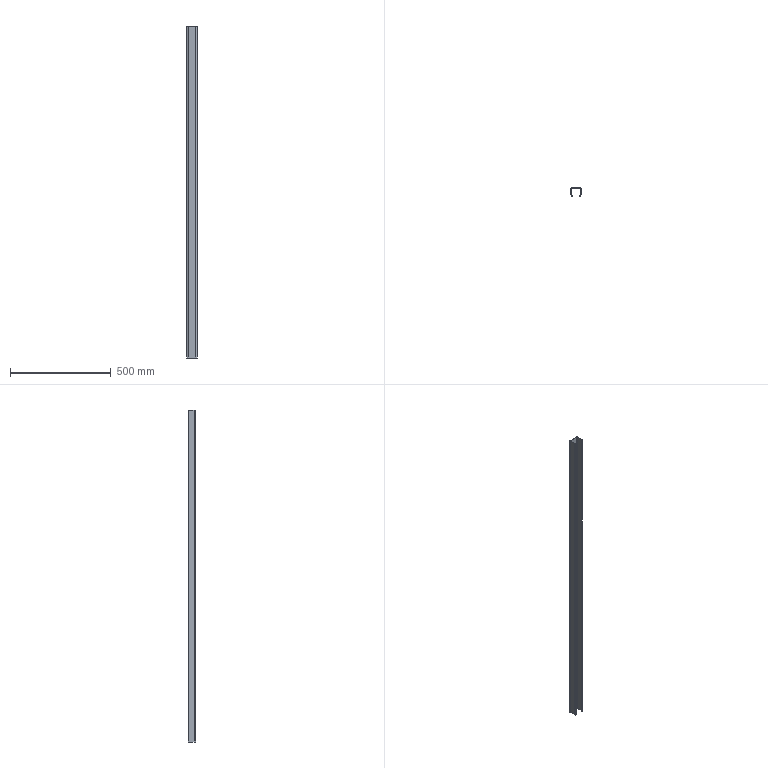Part | STEP file | 46A-00003CC12 | 1 solid | 28 faces | box 50 x 38.192 x 1650 mm | volume 271656 mm3 | plane 16 | cylinder 12 | commonest cylinder face diameters 1 x4 2 x4 4 x2 26 x2
STEP:
#1=CARTESIAN_POINT('',(27.525,37.856,-835.));
#2=VERTEX_POINT('',#1);
#3=CARTESIAN_POINT('',(28.525,38.856,-835.));
#4=VERTEX_POINT('',#3);
#5=CARTESIAN_POINT('',(27.525,37.856,-835.));
#6=CARTESIAN_POINT('',(27.525,37.954,-835.));
#7=CARTESIAN_POINT('',(27.537,38.052,-835.));
#8=CARTESIAN_POINT('',(27.561,38.148,-835.));
#9=CARTESIAN_POINT('',(27.632,38.332,-835.));
#10=CARTESIAN_POINT('',(27.745,38.494,-835.));
#11=CARTESIAN_POINT('',(27.812,38.567,-835.));
#12=CARTESIAN_POINT('',(27.961,38.696,-835.));
#13=CARTESIAN_POINT('',(28.137,38.786,-835.));
#14=CARTESIAN_POINT('',(28.23,38.819,-835.));
#15=CARTESIAN_POINT('',(28.346,38.846,-835.));
#16=CARTESIAN_POINT('',(28.464,38.855,-835.));
#17=CARTESIAN_POINT('',(28.484,38.856,-835.));
#18=CARTESIAN_POINT('',(28.505,38.856,-835.));
#19=CARTESIAN_POINT('',(28.525,38.856,-835.));
#20=B_SPLINE_CURVE_WITH_KNOTS('',5,(#5,#6,#7,#8,#9,#10,#11,#12,#13,#14,#15,#16,#17,#18,#19),.UNSPECIFIED.,.F.,.U.,(6,3,3,3,6),(0.,0.6928,1.386,2.078,2.221),.UNSPECIFIED.);
#21=EDGE_CURVE('',#2,#4,#20,.T.);
#22=ORIENTED_EDGE('',*,*,#21,.T.);
#23=CARTESIAN_POINT('',(76.525,38.856,-835.));
#24=VERTEX_POINT('',#23);
#25=CARTESIAN_POINT('',(52.525,38.856,-835.));
#26=DIRECTION('',(-1.,0.,0.));
#27=VECTOR('',#26,1.);
#28=LINE('',#25,#27);
#29=EDGE_CURVE('',#24,#4,#28,.T.);
#30=ORIENTED_EDGE('',*,*,#29,.F.);
#31=CARTESIAN_POINT('',(77.525,37.856,-835.));
#32=VERTEX_POINT('',#31);
#33=CARTESIAN_POINT('',(76.525,38.856,-835.));
#34=CARTESIAN_POINT('',(76.623,38.856,-835.));
#35=CARTESIAN_POINT('',(76.721,38.844,-835.));
#36=CARTESIAN_POINT('',(76.817,38.82,-835.));
#37=CARTESIAN_POINT('',(77.001,38.749,-835.));
#38=CARTESIAN_POINT('',(77.163,38.636,-835.));
#39=CARTESIAN_POINT('',(77.236,38.569,-835.));
#40=CARTESIAN_POINT('',(77.365,38.42,-835.));
#41=CARTESIAN_POINT('',(77.454,38.244,-835.));
#42=CARTESIAN_POINT('',(77.488,38.151,-835.));
#43=CARTESIAN_POINT('',(77.514,38.035,-835.));
#44=CARTESIAN_POINT('',(77.523,37.917,-835.));
#45=CARTESIAN_POINT('',(77.524,37.897,-835.));
#46=CARTESIAN_POINT('',(77.525,37.876,-835.));
#47=CARTESIAN_POINT('',(77.525,37.856,-835.));
#48=B_SPLINE_CURVE_WITH_KNOTS('',5,(#33,#34,#35,#36,#37,#38,#39,#40,#41,#42,#43,#44,#45,#46,#47),.UNSPECIFIED.,.F.,.U.,(6,3,3,3,6),(0.,0.6928,1.386,2.078,2.221),.UNSPECIFIED.);
#49=EDGE_CURVE('',#24,#32,#48,.T.);
#50=ORIENTED_EDGE('',*,*,#49,.T.);
#51=CARTESIAN_POINT('',(77.525,9.584,-835.));
#52=VERTEX_POINT('',#51);
#53=CARTESIAN_POINT('',(77.525,23.72,-835.));
#54=DIRECTION('',(0.,1.,0.));
#55=VECTOR('',#54,1.);
#56=LINE('',#53,#55);
#57=EDGE_CURVE('',#52,#32,#56,.T.);
#58=ORIENTED_EDGE('',*,*,#57,.F.);
#59=CARTESIAN_POINT('',(77.057,8.298,-835.));
#60=VERTEX_POINT('',#59);
#61=CARTESIAN_POINT('',(77.525,9.584,-835.));
#62=CARTESIAN_POINT('',(77.525,9.361,-835.));
#63=CARTESIAN_POINT('',(77.494,9.137,-835.));
#64=CARTESIAN_POINT('',(77.431,8.92,-835.));
#65=CARTESIAN_POINT('',(77.316,8.662,-835.));
#66=CARTESIAN_POINT('',(77.16,8.431,-835.));
#67=CARTESIAN_POINT('',(77.127,8.385,-835.));
#68=CARTESIAN_POINT('',(77.093,8.341,-835.));
#69=CARTESIAN_POINT('',(77.057,8.298,-835.));
#70=B_SPLINE_CURVE_WITH_KNOTS('',5,(#61,#62,#63,#64,#65,#66,#67,#68,#69),.UNSPECIFIED.,.F.,.U.,(6,3,6),(0.,1.58,1.974),.UNSPECIFIED.);
#71=EDGE_CURVE('',#52,#60,#70,.T.);
#72=ORIENTED_EDGE('',*,*,#71,.T.);
#73=CARTESIAN_POINT('',(72.768,3.187,-835.));
#74=VERTEX_POINT('',#73);
#75=CARTESIAN_POINT('',(74.912,5.743,-835.));
#76=DIRECTION('',(0.6428,0.766,0.));
#77=VECTOR('',#76,1.);
#78=LINE('',#75,#77);
#79=EDGE_CURVE('',#74,#60,#78,.T.);
#80=ORIENTED_EDGE('',*,*,#79,.F.);
#81=CARTESIAN_POINT('',(76.707,2.493,-835.));
#82=VERTEX_POINT('',#81);
#83=CARTESIAN_POINT('',(74.738,2.84,-835.));
#84=DIRECTION('',(-0.9848,0.1736,0.));
#85=VECTOR('',#84,1.);
#86=LINE('',#83,#85);
#87=EDGE_CURVE('',#82,#74,#86,.T.);
#88=ORIENTED_EDGE('',*,*,#87,.F.);
#89=CARTESIAN_POINT('',(72.397,0.6877,-835.));
#90=VERTEX_POINT('',#89);
#91=CARTESIAN_POINT('',(69.613,13.386,-835.));
#92=DIRECTION('',(0.,0.,1.));
#93=AXIS2_PLACEMENT_3D('',#91,#92,$);
#94=CIRCLE('',#93,13.);
#95=EDGE_CURVE('',#90,#82,#94,.T.);
#96=ORIENTED_EDGE('',*,*,#95,.F.);
#97=CARTESIAN_POINT('',(71.182,1.665,-835.));
#98=VERTEX_POINT('',#97);
#99=CARTESIAN_POINT('',(72.182,1.665,-835.));
#100=DIRECTION('',(0.,0.,1.));
#101=AXIS2_PLACEMENT_3D('',#99,#100,$);
#102=CIRCLE('',#101,1.);
#103=EDGE_CURVE('',#98,#90,#102,.T.);
#104=ORIENTED_EDGE('',*,*,#103,.F.);
#105=CARTESIAN_POINT('',(71.182,2.983,-835.));
#106=VERTEX_POINT('',#105);
#107=CARTESIAN_POINT('',(71.182,2.324,-835.));
#108=DIRECTION('',(0.,-1.,0.));
#109=VECTOR('',#108,1.);
#110=LINE('',#107,#109);
#111=EDGE_CURVE('',#106,#98,#110,.T.);
#112=ORIENTED_EDGE('',*,*,#111,.F.);
#113=CARTESIAN_POINT('',(71.299,3.304,-835.));
#114=VERTEX_POINT('',#113);
#115=CARTESIAN_POINT('',(71.182,2.983,-835.));
#116=CARTESIAN_POINT('',(71.182,3.038,-835.));
#117=CARTESIAN_POINT('',(71.19,3.094,-835.));
#118=CARTESIAN_POINT('',(71.206,3.149,-835.));
#119=CARTESIAN_POINT('',(71.235,3.213,-835.));
#120=CARTESIAN_POINT('',(71.274,3.271,-835.));
#121=CARTESIAN_POINT('',(71.282,3.282,-835.));
#122=CARTESIAN_POINT('',(71.29,3.293,-835.));
#123=CARTESIAN_POINT('',(71.299,3.304,-835.));
#124=B_SPLINE_CURVE_WITH_KNOTS('',5,(#115,#116,#117,#118,#119,#120,#121,#122,#123),.UNSPECIFIED.,.F.,.U.,(6,3,6),(0.,0.3949,0.4936),.UNSPECIFIED.);
#125=EDGE_CURVE('',#106,#114,#124,.T.);
#126=ORIENTED_EDGE('',*,*,#125,.T.);
#127=CARTESIAN_POINT('',(76.325,9.293,-835.));
#128=VERTEX_POINT('',#127);
#129=CARTESIAN_POINT('',(73.812,6.298,-835.));
#130=DIRECTION('',(-0.6428,-0.766,0.));
#131=VECTOR('',#130,1.);
#132=LINE('',#129,#131);
#133=EDGE_CURVE('',#128,#114,#132,.T.);
#134=ORIENTED_EDGE('',*,*,#133,.F.);
#135=CARTESIAN_POINT('',(76.325,37.156,-835.));
#136=VERTEX_POINT('',#135);
#137=CARTESIAN_POINT('',(76.325,23.225,-835.));
#138=DIRECTION('',(0.,-1.,0.));
#139=VECTOR('',#138,1.);
#140=LINE('',#137,#139);
#141=EDGE_CURVE('',#136,#128,#140,.T.);
#142=ORIENTED_EDGE('',*,*,#141,.F.);
#143=CARTESIAN_POINT('',(75.825,37.656,-835.));
#144=VERTEX_POINT('',#143);
#145=CARTESIAN_POINT('',(75.825,37.156,-835.));
#146=DIRECTION('',(0.,0.,1.));
#147=AXIS2_PLACEMENT_3D('',#145,#146,$);
#148=CIRCLE('',#147,0.5);
#149=EDGE_CURVE('',#136,#144,#148,.T.);
#150=ORIENTED_EDGE('',*,*,#149,.T.);
#151=CARTESIAN_POINT('',(29.225,37.656,-835.));
#152=VERTEX_POINT('',#151);
#153=CARTESIAN_POINT('',(52.525,37.656,-835.));
#154=DIRECTION('',(1.,0.,0.));
#155=VECTOR('',#154,1.);
#156=LINE('',#153,#155);
#157=EDGE_CURVE('',#152,#144,#156,.T.);
#158=ORIENTED_EDGE('',*,*,#157,.F.);
#159=CARTESIAN_POINT('',(28.725,37.156,-835.));
#160=VERTEX_POINT('',#159);
#161=CARTESIAN_POINT('',(29.225,37.156,-835.));
#162=DIRECTION('',(0.,0.,1.));
#163=AXIS2_PLACEMENT_3D('',#161,#162,$);
#164=CIRCLE('',#163,0.5);
#165=EDGE_CURVE('',#152,#160,#164,.T.);
#166=ORIENTED_EDGE('',*,*,#165,.T.);
#167=CARTESIAN_POINT('',(28.725,9.293,-835.));
#168=VERTEX_POINT('',#167);
#169=CARTESIAN_POINT('',(28.725,23.225,-835.));
#170=DIRECTION('',(0.,1.,0.));
#171=VECTOR('',#170,1.);
#172=LINE('',#169,#171);
#173=EDGE_CURVE('',#168,#160,#172,.T.);
#174=ORIENTED_EDGE('',*,*,#173,.F.);
#175=CARTESIAN_POINT('',(33.75,3.304,-835.));
#176=VERTEX_POINT('',#175);
#177=CARTESIAN_POINT('',(31.237,6.298,-835.));
#178=DIRECTION('',(-0.6428,0.766,0.));
#179=VECTOR('',#178,1.);
#180=LINE('',#177,#179);
#181=EDGE_CURVE('',#176,#168,#180,.T.);
#182=ORIENTED_EDGE('',*,*,#181,.F.);
#183=CARTESIAN_POINT('',(33.867,2.983,-835.));
#184=VERTEX_POINT('',#183);
#185=CARTESIAN_POINT('',(33.75,3.304,-835.));
#186=CARTESIAN_POINT('',(33.786,3.261,-835.));
#187=CARTESIAN_POINT('',(33.816,3.213,-835.));
#188=CARTESIAN_POINT('',(33.839,3.162,-835.));
#189=CARTESIAN_POINT('',(33.858,3.094,-835.));
#190=CARTESIAN_POINT('',(33.866,3.024,-835.));
#191=CARTESIAN_POINT('',(33.867,3.01,-835.));
#192=CARTESIAN_POINT('',(33.867,2.997,-835.));
#193=CARTESIAN_POINT('',(33.867,2.983,-835.));
#194=B_SPLINE_CURVE_WITH_KNOTS('',5,(#185,#186,#187,#188,#189,#190,#191,#192,#193),.UNSPECIFIED.,.F.,.U.,(6,3,6),(0.,0.3949,0.4936),.UNSPECIFIED.);
#195=EDGE_CURVE('',#176,#184,#194,.T.);
#196=ORIENTED_EDGE('',*,*,#195,.T.);
#197=CARTESIAN_POINT('',(33.867,1.665,-835.));
#198=VERTEX_POINT('',#197);
#199=CARTESIAN_POINT('',(33.867,2.324,-835.));
#200=DIRECTION('',(0.,1.,0.));
#201=VECTOR('',#200,1.);
#202=LINE('',#199,#201);
#203=EDGE_CURVE('',#198,#184,#202,.T.);
#204=ORIENTED_EDGE('',*,*,#203,.F.);
#205=CARTESIAN_POINT('',(32.653,0.6877,-835.));
#206=VERTEX_POINT('',#205);
#207=CARTESIAN_POINT('',(32.867,1.665,-835.));
#208=DIRECTION('',(0.,0.,1.));
#209=AXIS2_PLACEMENT_3D('',#207,#208,$);
#210=CIRCLE('',#209,1.);
#211=EDGE_CURVE('',#206,#198,#210,.T.);
#212=ORIENTED_EDGE('',*,*,#211,.F.);
#213=CARTESIAN_POINT('',(28.342,2.493,-835.));
#214=VERTEX_POINT('',#213);
#215=CARTESIAN_POINT('',(35.437,13.386,-835.));
#216=DIRECTION('',(0.,0.,1.));
#217=AXIS2_PLACEMENT_3D('',#215,#216,$);
#218=CIRCLE('',#217,13.);
#219=EDGE_CURVE('',#214,#206,#218,.T.);
#220=ORIENTED_EDGE('',*,*,#219,.F.);
#221=CARTESIAN_POINT('',(32.281,3.187,-835.));
#222=VERTEX_POINT('',#221);
#223=CARTESIAN_POINT('',(30.312,2.84,-835.));
#224=DIRECTION('',(-0.9848,-0.1736,0.));
#225=VECTOR('',#224,1.);
#226=LINE('',#223,#225);
#227=EDGE_CURVE('',#222,#214,#226,.T.);
#228=ORIENTED_EDGE('',*,*,#227,.F.);
#229=CARTESIAN_POINT('',(27.993,8.298,-835.));
#230=VERTEX_POINT('',#229);
#231=CARTESIAN_POINT('',(30.137,5.743,-835.));
#232=DIRECTION('',(0.6428,-0.766,0.));
#233=VECTOR('',#232,1.);
#234=LINE('',#231,#233);
#235=EDGE_CURVE('',#230,#222,#234,.T.);
#236=ORIENTED_EDGE('',*,*,#235,.F.);
#237=CARTESIAN_POINT('',(27.525,9.584,-835.));
#238=VERTEX_POINT('',#237);
#239=CARTESIAN_POINT('',(27.993,8.298,-835.));
#240=CARTESIAN_POINT('',(27.849,8.47,-835.));
#241=CARTESIAN_POINT('',(27.729,8.661,-835.));
#242=CARTESIAN_POINT('',(27.637,8.868,-835.));
#243=CARTESIAN_POINT('',(27.56,9.139,-835.));
#244=CARTESIAN_POINT('',(27.531,9.417,-835.));
#245=CARTESIAN_POINT('',(27.527,9.472,-835.));
#246=CARTESIAN_POINT('',(27.525,9.528,-835.));
#247=CARTESIAN_POINT('',(27.525,9.584,-835.));
#248=B_SPLINE_CURVE_WITH_KNOTS('',5,(#239,#240,#241,#242,#243,#244,#245,#246,#247),.UNSPECIFIED.,.F.,.U.,(6,3,6),(0.,1.58,1.974),.UNSPECIFIED.);
#249=EDGE_CURVE('',#230,#238,#248,.T.);
#250=ORIENTED_EDGE('',*,*,#249,.T.);
#251=CARTESIAN_POINT('',(27.525,23.72,-835.));
#252=DIRECTION('',(0.,-1.,0.));
#253=VECTOR('',#252,1.);
#254=LINE('',#251,#253);
#255=EDGE_CURVE('',#2,#238,#254,.T.);
#256=ORIENTED_EDGE('',*,*,#255,.F.);
#257=EDGE_LOOP('',(#22,#30,#50,#58,#72,#80,#88,#96,#104,#112,#126,#134,#142,#150,#158,#166,#174,#182,#196,#204,#212,#220,#228,#236,#250,#256));
#258=FACE_OUTER_BOUND('',#257,.T.);
#259=CARTESIAN_POINT('',(35.437,13.386,-835.));
#260=DIRECTION('',(0.,0.,1.));
#261=DIRECTION('',(1.,0.,0.));
#262=AXIS2_PLACEMENT_3D('',#259,#260,#261);
#263=PLANE('',#262);
#264=ADVANCED_FACE('',(#258),#263,.F.);
#265=CARTESIAN_POINT('',(77.525,37.856,815.));
#266=VERTEX_POINT('',#265);
#267=CARTESIAN_POINT('',(77.525,37.856,835.));
#268=DIRECTION('',(0.,0.,-1.));
#269=VECTOR('',#268,1.);
#270=LINE('',#267,#269);
#271=EDGE_CURVE('',#32,#266,#270,.F.);
#272=ORIENTED_EDGE('',*,*,#271,.F.);
#273=ORIENTED_EDGE('',*,*,#49,.F.);
#274=CARTESIAN_POINT('',(76.525,38.856,815.));
#275=VERTEX_POINT('',#274);
#276=CARTESIAN_POINT('',(76.525,38.856,835.));
#277=DIRECTION('',(0.,0.,-1.));
#278=VECTOR('',#277,1.);
#279=LINE('',#276,#278);
#280=EDGE_CURVE('',#275,#24,#279,.T.);
#281=ORIENTED_EDGE('',*,*,#280,.F.);
#282=CARTESIAN_POINT('',(76.525,37.856,815.));
#283=DIRECTION('',(0.,0.,-1.));
#284=AXIS2_PLACEMENT_3D('',#282,#283,$);
#285=CIRCLE('',#284,1.);
#286=EDGE_CURVE('',#275,#266,#285,.T.);
#287=ORIENTED_EDGE('',*,*,#286,.T.);
#288=EDGE_LOOP('',(#272,#273,#281,#287));
#289=FACE_OUTER_BOUND('',#288,.T.);
#290=CARTESIAN_POINT('',(76.525,37.856,835.));
#291=DIRECTION('',(0.,0.,-1.));
#292=DIRECTION('',(-1.,0.,0.));
#293=AXIS2_PLACEMENT_3D('',#290,#291,#292);
#294=CYLINDRICAL_SURFACE('',#293,1.);
#295=ADVANCED_FACE('',(#289),#294,.T.);
#296=CARTESIAN_POINT('',(77.525,9.584,815.));
#297=VERTEX_POINT('',#296);
#298=CARTESIAN_POINT('',(77.525,23.72,815.));
#299=DIRECTION('',(0.,1.,0.));
#300=VECTOR('',#299,1.);
#301=LINE('',#298,#300);
#302=EDGE_CURVE('',#297,#266,#301,.T.);
#303=ORIENTED_EDGE('',*,*,#302,.F.);
#304=CARTESIAN_POINT('',(77.525,9.584,-10.));
#305=DIRECTION('',(0.,0.,-1.));
#306=VECTOR('',#305,1.);
#307=LINE('',#304,#306);
#308=EDGE_CURVE('',#297,#52,#307,.T.);
#309=ORIENTED_EDGE('',*,*,#308,.T.);
#310=ORIENTED_EDGE('',*,*,#57,.T.);
#311=ORIENTED_EDGE('',*,*,#271,.T.);
#312=EDGE_LOOP('',(#303,#309,#310,#311));
#313=FACE_OUTER_BOUND('',#312,.T.);
#314=CARTESIAN_POINT('',(77.525,8.856,835.));
#315=DIRECTION('',(-1.,0.,0.));
#316=DIRECTION('',(0.,0.,1.));
#317=AXIS2_PLACEMENT_3D('',#314,#315,#316);
#318=PLANE('',#317);
#319=ADVANCED_FACE('',(#313),#318,.F.);
#320=ORIENTED_EDGE('',*,*,#308,.F.);
#321=CARTESIAN_POINT('',(77.057,8.298,815.));
#322=VERTEX_POINT('',#321);
#323=CARTESIAN_POINT('',(75.525,9.584,815.));
#324=DIRECTION('',(0.,0.,-1.));
#325=AXIS2_PLACEMENT_3D('',#323,#324,$);
#326=CIRCLE('',#325,2.);
#327=EDGE_CURVE('',#322,#297,#326,.F.);
#328=ORIENTED_EDGE('',*,*,#327,.F.);
#329=CARTESIAN_POINT('',(77.057,8.298,835.));
#330=DIRECTION('',(0.,0.,-1.));
#331=VECTOR('',#330,1.);
#332=LINE('',#329,#331);
#333=EDGE_CURVE('',#60,#322,#332,.F.);
#334=ORIENTED_EDGE('',*,*,#333,.F.);
#335=ORIENTED_EDGE('',*,*,#71,.F.);
#336=EDGE_LOOP('',(#320,#328,#334,#335));
#337=FACE_OUTER_BOUND('',#336,.T.);
#338=CARTESIAN_POINT('',(75.525,9.584,835.));
#339=DIRECTION('',(0.,0.,-1.));
#340=DIRECTION('',(1.,0.,0.));
#341=AXIS2_PLACEMENT_3D('',#338,#339,#340);
#342=CYLINDRICAL_SURFACE('',#341,2.);
#343=ADVANCED_FACE('',(#337),#342,.T.);
#344=CARTESIAN_POINT('',(72.768,3.187,815.));
#345=VERTEX_POINT('',#344);
#346=CARTESIAN_POINT('',(74.912,5.743,815.));
#347=DIRECTION('',(0.6428,0.766,0.));
#348=VECTOR('',#347,1.);
#349=LINE('',#346,#348);
#350=EDGE_CURVE('',#345,#322,#349,.T.);
#351=ORIENTED_EDGE('',*,*,#350,.F.);
#352=CARTESIAN_POINT('',(72.768,3.187,-10.));
#353=DIRECTION('',(0.,0.,-1.));
#354=VECTOR('',#353,1.);
#355=LINE('',#352,#354);
#356=EDGE_CURVE('',#345,#74,#355,.T.);
#357=ORIENTED_EDGE('',*,*,#356,.T.);
#358=ORIENTED_EDGE('',*,*,#79,.T.);
#359=ORIENTED_EDGE('',*,*,#333,.T.);
#360=EDGE_LOOP('',(#351,#357,#358,#359));
#361=FACE_OUTER_BOUND('',#360,.T.);
#362=CARTESIAN_POINT('',(77.525,8.856,835.));
#363=DIRECTION('',(-0.766,0.6428,0.));
#364=DIRECTION('',(-0.6428,-0.766,0.));
#365=AXIS2_PLACEMENT_3D('',#362,#363,#364);
#366=PLANE('',#365);
#367=ADVANCED_FACE('',(#361),#366,.F.);
#368=ORIENTED_EDGE('',*,*,#356,.F.);
#369=CARTESIAN_POINT('',(76.707,2.493,815.));
#370=VERTEX_POINT('',#369);
#371=CARTESIAN_POINT('',(74.738,2.84,815.));
#372=DIRECTION('',(-0.9848,0.1736,0.));
#373=VECTOR('',#372,1.);
#374=LINE('',#371,#373);
#375=EDGE_CURVE('',#370,#345,#374,.T.);
#376=ORIENTED_EDGE('',*,*,#375,.F.);
#377=CARTESIAN_POINT('',(76.707,2.493,-10.));
#378=DIRECTION('',(0.,0.,-1.));
#379=VECTOR('',#378,1.);
#380=LINE('',#377,#379);
#381=EDGE_CURVE('',#370,#82,#380,.T.);
#382=ORIENTED_EDGE('',*,*,#381,.T.);
#383=ORIENTED_EDGE('',*,*,#87,.T.);
#384=EDGE_LOOP('',(#368,#376,#382,#383));
#385=FACE_OUTER_BOUND('',#384,.T.);
#386=CARTESIAN_POINT('',(72.768,3.187,835.));
#387=DIRECTION('',(-0.1736,-0.9848,0.));
#388=DIRECTION('',(0.9848,-0.1736,0.));
#389=AXIS2_PLACEMENT_3D('',#386,#387,#388);
#390=PLANE('',#389);
#391=ADVANCED_FACE('',(#385),#390,.F.);
#392=ORIENTED_EDGE('',*,*,#95,.T.);
#393=ORIENTED_EDGE('',*,*,#381,.F.);
#394=CARTESIAN_POINT('',(72.397,0.6877,815.));
#395=VERTEX_POINT('',#394);
#396=CARTESIAN_POINT('',(69.613,13.386,815.));
#397=DIRECTION('',(0.,0.,-1.));
#398=AXIS2_PLACEMENT_3D('',#396,#397,$);
#399=CIRCLE('',#398,13.);
#400=EDGE_CURVE('',#395,#370,#399,.F.);
#401=ORIENTED_EDGE('',*,*,#400,.F.);
#402=CARTESIAN_POINT('',(72.397,0.6877,835.));
#403=DIRECTION('',(0.,0.,-1.));
#404=VECTOR('',#403,1.);
#405=LINE('',#402,#404);
#406=EDGE_CURVE('',#395,#90,#405,.T.);
#407=ORIENTED_EDGE('',*,*,#406,.T.);
#408=EDGE_LOOP('',(#392,#393,#401,#407));
#409=FACE_OUTER_BOUND('',#408,.T.);
#410=CARTESIAN_POINT('',(69.613,13.386,835.));
#411=DIRECTION('',(0.,0.,-1.));
#412=DIRECTION('',(1.,0.,0.));
#413=AXIS2_PLACEMENT_3D('',#410,#411,#412);
#414=CYLINDRICAL_SURFACE('',#413,13.);
#415=ADVANCED_FACE('',(#409),#414,.T.);
#416=ORIENTED_EDGE('',*,*,#406,.F.);
#417=CARTESIAN_POINT('',(71.182,1.665,815.));
#418=VERTEX_POINT('',#417);
#419=CARTESIAN_POINT('',(72.182,1.665,815.));
#420=DIRECTION('',(0.,0.,-1.));
#421=AXIS2_PLACEMENT_3D('',#419,#420,$);
#422=CIRCLE('',#421,1.);
#423=EDGE_CURVE('',#418,#395,#422,.F.);
#424=ORIENTED_EDGE('',*,*,#423,.F.);
#425=CARTESIAN_POINT('',(71.182,1.665,835.));
#426=DIRECTION('',(0.,0.,-1.));
#427=VECTOR('',#426,1.);
#428=LINE('',#425,#427);
#429=EDGE_CURVE('',#418,#98,#428,.T.);
#430=ORIENTED_EDGE('',*,*,#429,.T.);
#431=ORIENTED_EDGE('',*,*,#103,.T.);
#432=EDGE_LOOP('',(#416,#424,#430,#431));
#433=FACE_OUTER_BOUND('',#432,.T.);
#434=CARTESIAN_POINT('',(72.182,1.665,835.));
#435=DIRECTION('',(0.,0.,-1.));
#436=DIRECTION('',(1.,0.,0.));
#437=AXIS2_PLACEMENT_3D('',#434,#435,#436);
#438=CYLINDRICAL_SURFACE('',#437,1.);
#439=ADVANCED_FACE('',(#433),#438,.T.);
#440=CARTESIAN_POINT('',(71.182,2.983,815.));
#441=VERTEX_POINT('',#440);
#442=CARTESIAN_POINT('',(71.182,2.324,815.));
#443=DIRECTION('',(0.,-1.,0.));
#444=VECTOR('',#443,1.);
#445=LINE('',#442,#444);
#446=EDGE_CURVE('',#441,#418,#445,.T.);
#447=ORIENTED_EDGE('',*,*,#446,.F.);
#448=CARTESIAN_POINT('',(71.182,2.983,-10.));
#449=DIRECTION('',(0.,0.,-1.));
#450=VECTOR('',#449,1.);
#451=LINE('',#448,#450);
#452=EDGE_CURVE('',#441,#106,#451,.T.);
#453=ORIENTED_EDGE('',*,*,#452,.T.);
#454=ORIENTED_EDGE('',*,*,#111,.T.);
#455=ORIENTED_EDGE('',*,*,#429,.F.);
#456=EDGE_LOOP('',(#447,#453,#454,#455));
#457=FACE_OUTER_BOUND('',#456,.T.);
#458=CARTESIAN_POINT('',(71.182,1.665,835.));
#459=DIRECTION('',(1.,0.,0.));
#460=DIRECTION('',(0.,0.,-1.));
#461=AXIS2_PLACEMENT_3D('',#458,#459,#460);
#462=PLANE('',#461);
#463=ADVANCED_FACE('',(#457),#462,.F.);
#464=ORIENTED_EDGE('',*,*,#452,.F.);
#465=CARTESIAN_POINT('',(71.299,3.304,815.));
#466=VERTEX_POINT('',#465);
#467=CARTESIAN_POINT('',(71.682,2.983,815.));
#468=DIRECTION('',(0.,0.,-1.));
#469=AXIS2_PLACEMENT_3D('',#467,#468,$);
#470=CIRCLE('',#469,0.5);
#471=EDGE_CURVE('',#466,#441,#470,.F.);
#472=ORIENTED_EDGE('',*,*,#471,.F.);
#473=CARTESIAN_POINT('',(71.299,3.304,835.));
#474=DIRECTION('',(0.,0.,-1.));
#475=VECTOR('',#474,1.);
#476=LINE('',#473,#475);
#477=EDGE_CURVE('',#114,#466,#476,.F.);
#478=ORIENTED_EDGE('',*,*,#477,.F.);
#479=ORIENTED_EDGE('',*,*,#125,.F.);
#480=EDGE_LOOP('',(#464,#472,#478,#479));
#481=FACE_OUTER_BOUND('',#480,.T.);
#482=CARTESIAN_POINT('',(71.682,2.983,835.));
#483=DIRECTION('',(0.,0.,-1.));
#484=DIRECTION('',(-1.,0.,0.));
#485=AXIS2_PLACEMENT_3D('',#482,#483,#484);
#486=CYLINDRICAL_SURFACE('',#485,0.5);
#487=ADVANCED_FACE('',(#481),#486,.T.);
#488=CARTESIAN_POINT('',(76.325,9.293,815.));
#489=VERTEX_POINT('',#488);
#490=CARTESIAN_POINT('',(73.812,6.298,815.));
#491=DIRECTION('',(-0.6428,-0.766,0.));
#492=VECTOR('',#491,1.);
#493=LINE('',#490,#492);
#494=EDGE_CURVE('',#489,#466,#493,.T.);
#495=ORIENTED_EDGE('',*,*,#494,.F.);
#496=CARTESIAN_POINT('',(76.325,9.293,-10.));
#497=DIRECTION('',(0.,0.,-1.));
#498=VECTOR('',#497,1.);
#499=LINE('',#496,#498);
#500=EDGE_CURVE('',#489,#128,#499,.T.);
#501=ORIENTED_EDGE('',*,*,#500,.T.);
#502=ORIENTED_EDGE('',*,*,#133,.T.);
#503=ORIENTED_EDGE('',*,*,#477,.T.);
#504=EDGE_LOOP('',(#495,#501,#502,#503));
#505=FACE_OUTER_BOUND('',#504,.T.);
#506=CARTESIAN_POINT('',(76.325,9.293,835.));
#507=DIRECTION('',(0.766,-0.6428,0.));
#508=DIRECTION('',(0.6428,0.766,0.));
#509=AXIS2_PLACEMENT_3D('',#506,#507,#508);
#510=PLANE('',#509);
#511=ADVANCED_FACE('',(#505),#510,.F.);
#512=ORIENTED_EDGE('',*,*,#500,.F.);
#513=CARTESIAN_POINT('',(76.325,37.156,815.));
#514=VERTEX_POINT('',#513);
#515=CARTESIAN_POINT('',(76.325,23.225,815.));
#516=DIRECTION('',(0.,-1.,0.));
#517=VECTOR('',#516,1.);
#518=LINE('',#515,#517);
#519=EDGE_CURVE('',#514,#489,#518,.T.);
#520=ORIENTED_EDGE('',*,*,#519,.F.);
#521=CARTESIAN_POINT('',(76.325,37.156,-10.));
#522=DIRECTION('',(0.,0.,-1.));
#523=VECTOR('',#522,1.);
#524=LINE('',#521,#523);
#525=EDGE_CURVE('',#514,#136,#524,.T.);
#526=ORIENTED_EDGE('',*,*,#525,.T.);
#527=ORIENTED_EDGE('',*,*,#141,.T.);
#528=EDGE_LOOP('',(#512,#520,#526,#527));
#529=FACE_OUTER_BOUND('',#528,.T.);
#530=CARTESIAN_POINT('',(76.325,9.293,835.));
#531=DIRECTION('',(1.,0.,0.));
#532=DIRECTION('',(0.,1.,0.));
#533=AXIS2_PLACEMENT_3D('',#530,#531,#532);
#534=PLANE('',#533);
#535=ADVANCED_FACE('',(#529),#534,.F.);
#536=CARTESIAN_POINT('',(75.825,37.656,815.));
#537=VERTEX_POINT('',#536);
#538=CARTESIAN_POINT('',(75.825,37.156,815.));
#539=DIRECTION('',(0.,0.,1.));
#540=AXIS2_PLACEMENT_3D('',#538,#539,$);
#541=CIRCLE('',#540,0.5);
#542=EDGE_CURVE('',#537,#514,#541,.F.);
#543=ORIENTED_EDGE('',*,*,#542,.F.);
#544=CARTESIAN_POINT('',(75.825,37.656,835.));
#545=DIRECTION('',(0.,0.,1.));
#546=VECTOR('',#545,1.);
#547=LINE('',#544,#546);
#548=EDGE_CURVE('',#144,#537,#547,.T.);
#549=ORIENTED_EDGE('',*,*,#548,.F.);
#550=ORIENTED_EDGE('',*,*,#149,.F.);
#551=ORIENTED_EDGE('',*,*,#525,.F.);
#552=EDGE_LOOP('',(#543,#549,#550,#551));
#553=FACE_OUTER_BOUND('',#552,.T.);
#554=CARTESIAN_POINT('',(75.825,37.156,835.));
#555=DIRECTION('',(0.,0.,1.));
#556=DIRECTION('',(1.,0.,0.));
#557=AXIS2_PLACEMENT_3D('',#554,#555,#556);
#558=CYLINDRICAL_SURFACE('',#557,0.5);
#559=ADVANCED_FACE('',(#553),#558,.F.);
#560=CARTESIAN_POINT('',(29.225,37.656,815.));
#561=VERTEX_POINT('',#560);
#562=CARTESIAN_POINT('',(52.525,37.656,815.));
#563=DIRECTION('',(1.,0.,0.));
#564=VECTOR('',#563,1.);
#565=LINE('',#562,#564);
#566=EDGE_CURVE('',#561,#537,#565,.T.);
#567=ORIENTED_EDGE('',*,*,#566,.F.);
#568=CARTESIAN_POINT('',(29.225,37.656,-10.));
#569=DIRECTION('',(0.,0.,-1.));
#570=VECTOR('',#569,1.);
#571=LINE('',#568,#570);
#572=EDGE_CURVE('',#561,#152,#571,.T.);
#573=ORIENTED_EDGE('',*,*,#572,.T.);
#574=ORIENTED_EDGE('',*,*,#157,.T.);
#575=ORIENTED_EDGE('',*,*,#548,.T.);
#576=EDGE_LOOP('',(#567,#573,#574,#575));
#577=FACE_OUTER_BOUND('',#576,.T.);
#578=CARTESIAN_POINT('',(28.725,37.656,835.));
#579=DIRECTION('',(0.,1.,0.));
#580=DIRECTION('',(-1.,0.,0.));
#581=AXIS2_PLACEMENT_3D('',#578,#579,#580);
#582=PLANE('',#581);
#583=ADVANCED_FACE('',(#577),#582,.F.);
#584=CARTESIAN_POINT('',(28.725,37.156,815.));
#585=VERTEX_POINT('',#584);
#586=CARTESIAN_POINT('',(29.225,37.156,815.));
#587=DIRECTION('',(0.,0.,1.));
#588=AXIS2_PLACEMENT_3D('',#586,#587,$);
#589=CIRCLE('',#588,0.5);
#590=EDGE_CURVE('',#585,#561,#589,.F.);
#591=ORIENTED_EDGE('',*,*,#590,.F.);
#592=CARTESIAN_POINT('',(28.725,37.156,835.));
#593=DIRECTION('',(0.,0.,1.));
#594=VECTOR('',#593,1.);
#595=LINE('',#592,#594);
#596=EDGE_CURVE('',#160,#585,#595,.T.);
#597=ORIENTED_EDGE('',*,*,#596,.F.);
#598=ORIENTED_EDGE('',*,*,#165,.F.);
#599=ORIENTED_EDGE('',*,*,#572,.F.);
#600=EDGE_LOOP('',(#591,#597,#598,#599));
#601=FACE_OUTER_BOUND('',#600,.T.);
#602=CARTESIAN_POINT('',(29.225,37.156,835.));
#603=DIRECTION('',(0.,0.,1.));
#604=DIRECTION('',(1.,0.,0.));
#605=AXIS2_PLACEMENT_3D('',#602,#603,#604);
#606=CYLINDRICAL_SURFACE('',#605,0.5);
#607=ADVANCED_FACE('',(#601),#606,.F.);
#608=CARTESIAN_POINT('',(28.725,9.293,815.));
#609=VERTEX_POINT('',#608);
#610=CARTESIAN_POINT('',(28.725,23.225,815.));
#611=DIRECTION('',(0.,1.,0.));
#612=VECTOR('',#611,1.);
#613=LINE('',#610,#612);
#614=EDGE_CURVE('',#609,#585,#613,.T.);
#615=ORIENTED_EDGE('',*,*,#614,.F.);
#616=CARTESIAN_POINT('',(28.725,9.293,-10.));
#617=DIRECTION('',(0.,0.,-1.));
#618=VECTOR('',#617,1.);
#619=LINE('',#616,#618);
#620=EDGE_CURVE('',#609,#168,#619,.T.);
#621=ORIENTED_EDGE('',*,*,#620,.T.);
#622=ORIENTED_EDGE('',*,*,#173,.T.);
#623=ORIENTED_EDGE('',*,*,#596,.T.);
#624=EDGE_LOOP('',(#615,#621,#622,#623));
#625=FACE_OUTER_BOUND('',#624,.T.);
#626=CARTESIAN_POINT('',(28.725,9.293,835.));
#627=DIRECTION('',(-1.,0.,0.));
#628=DIRECTION('',(0.,0.,1.));
#629=AXIS2_PLACEMENT_3D('',#626,#627,#628);
#630=PLANE('',#629);
#631=ADVANCED_FACE('',(#625),#630,.F.);
#632=ORIENTED_EDGE('',*,*,#620,.F.);
#633=CARTESIAN_POINT('',(33.75,3.304,815.));
#634=VERTEX_POINT('',#633);
#635=CARTESIAN_POINT('',(31.237,6.298,815.));
#636=DIRECTION('',(-0.6428,0.766,0.));
#637=VECTOR('',#636,1.);
#638=LINE('',#635,#637);
#639=EDGE_CURVE('',#634,#609,#638,.T.);
#640=ORIENTED_EDGE('',*,*,#639,.F.);
#641=CARTESIAN_POINT('',(33.75,3.304,-10.));
#642=DIRECTION('',(0.,0.,-1.));
#643=VECTOR('',#642,1.);
#644=LINE('',#641,#643);
#645=EDGE_CURVE('',#634,#176,#644,.T.);
#646=ORIENTED_EDGE('',*,*,#645,.T.);
#647=ORIENTED_EDGE('',*,*,#181,.T.);
#648=EDGE_LOOP('',(#632,#640,#646,#647));
#649=FACE_OUTER_BOUND('',#648,.T.);
#650=CARTESIAN_POINT('',(28.725,9.293,835.));
#651=DIRECTION('',(-0.766,-0.6428,0.));
#652=DIRECTION('',(0.6428,-0.766,0.));
#653=AXIS2_PLACEMENT_3D('',#650,#651,#652);
#654=PLANE('',#653);
#655=ADVANCED_FACE('',(#649),#654,.F.);
#656=ORIENTED_EDGE('',*,*,#645,.F.);
#657=CARTESIAN_POINT('',(33.867,2.983,815.));
#658=VERTEX_POINT('',#657);
#659=CARTESIAN_POINT('',(33.367,2.983,815.));
#660=DIRECTION('',(0.,0.,-1.));
#661=AXIS2_PLACEMENT_3D('',#659,#660,$);
#662=CIRCLE('',#661,0.5);
#663=EDGE_CURVE('',#658,#634,#662,.F.);
#664=ORIENTED_EDGE('',*,*,#663,.F.);
#665=CARTESIAN_POINT('',(33.867,2.983,835.));
#666=DIRECTION('',(0.,0.,-1.));
#667=VECTOR('',#666,1.);
#668=LINE('',#665,#667);
#669=EDGE_CURVE('',#184,#658,#668,.F.);
#670=ORIENTED_EDGE('',*,*,#669,.F.);
#671=ORIENTED_EDGE('',*,*,#195,.F.);
#672=EDGE_LOOP('',(#656,#664,#670,#671));
#673=FACE_OUTER_BOUND('',#672,.T.);
#674=CARTESIAN_POINT('',(33.367,2.983,835.));
#675=DIRECTION('',(0.,0.,-1.));
#676=DIRECTION('',(-1.,0.,0.));
#677=AXIS2_PLACEMENT_3D('',#674,#675,#676);
#678=CYLINDRICAL_SURFACE('',#677,0.5);
#679=ADVANCED_FACE('',(#673),#678,.T.);
#680=CARTESIAN_POINT('',(33.867,1.665,815.));
#681=VERTEX_POINT('',#680);
#682=CARTESIAN_POINT('',(33.867,2.324,815.));
#683=DIRECTION('',(0.,1.,0.));
#684=VECTOR('',#683,1.);
#685=LINE('',#682,#684);
#686=EDGE_CURVE('',#681,#658,#685,.T.);
#687=ORIENTED_EDGE('',*,*,#686,.F.);
#688=CARTESIAN_POINT('',(33.867,1.665,-10.));
#689=DIRECTION('',(0.,0.,-1.));
#690=VECTOR('',#689,1.);
#691=LINE('',#688,#690);
#692=EDGE_CURVE('',#681,#198,#691,.T.);
#693=ORIENTED_EDGE('',*,*,#692,.T.);
#694=ORIENTED_EDGE('',*,*,#203,.T.);
#695=ORIENTED_EDGE('',*,*,#669,.T.);
#696=EDGE_LOOP('',(#687,#693,#694,#695));
#697=FACE_OUTER_BOUND('',#696,.T.);
#698=CARTESIAN_POINT('',(33.867,1.665,835.));
#699=DIRECTION('',(-1.,0.,0.));
#700=DIRECTION('',(0.,0.,1.));
#701=AXIS2_PLACEMENT_3D('',#698,#699,#700);
#702=PLANE('',#701);
#703=ADVANCED_FACE('',(#697),#702,.F.);
#704=ORIENTED_EDGE('',*,*,#692,.F.);
#705=CARTESIAN_POINT('',(32.653,0.6877,815.));
#706=VERTEX_POINT('',#705);
#707=CARTESIAN_POINT('',(32.867,1.665,815.));
#708=DIRECTION('',(0.,0.,-1.));
#709=AXIS2_PLACEMENT_3D('',#707,#708,$);
#710=CIRCLE('',#709,1.);
#711=EDGE_CURVE('',#706,#681,#710,.F.);
#712=ORIENTED_EDGE('',*,*,#711,.F.);
#713=CARTESIAN_POINT('',(32.653,0.6877,835.));
#714=DIRECTION('',(0.,0.,-1.));
#715=VECTOR('',#714,1.);
#716=LINE('',#713,#715);
#717=EDGE_CURVE('',#706,#206,#716,.T.);
#718=ORIENTED_EDGE('',*,*,#717,.T.);
#719=ORIENTED_EDGE('',*,*,#211,.T.);
#720=EDGE_LOOP('',(#704,#712,#718,#719));
#721=FACE_OUTER_BOUND('',#720,.T.);
#722=CARTESIAN_POINT('',(32.867,1.665,835.));
#723=DIRECTION('',(0.,0.,-1.));
#724=DIRECTION('',(1.,0.,0.));
#725=AXIS2_PLACEMENT_3D('',#722,#723,#724);
#726=CYLINDRICAL_SURFACE('',#725,1.);
#727=ADVANCED_FACE('',(#721),#726,.T.);
#728=ORIENTED_EDGE('',*,*,#717,.F.);
#729=CARTESIAN_POINT('',(28.342,2.493,815.));
#730=VERTEX_POINT('',#729);
#731=CARTESIAN_POINT('',(35.437,13.386,815.));
#732=DIRECTION('',(0.,0.,-1.));
#733=AXIS2_PLACEMENT_3D('',#731,#732,$);
#734=CIRCLE('',#733,13.);
#735=EDGE_CURVE('',#730,#706,#734,.F.);
#736=ORIENTED_EDGE('',*,*,#735,.F.);
#737=CARTESIAN_POINT('',(28.342,2.493,835.));
#738=DIRECTION('',(0.,0.,-1.));
#739=VECTOR('',#738,1.);
#740=LINE('',#737,#739);
#741=EDGE_CURVE('',#730,#214,#740,.T.);
#742=ORIENTED_EDGE('',*,*,#741,.T.);
#743=ORIENTED_EDGE('',*,*,#219,.T.);
#744=EDGE_LOOP('',(#728,#736,#742,#743));
#745=FACE_OUTER_BOUND('',#744,.T.);
#746=CARTESIAN_POINT('',(35.437,13.386,835.));
#747=DIRECTION('',(0.,0.,-1.));
#748=DIRECTION('',(1.,0.,0.));
#749=AXIS2_PLACEMENT_3D('',#746,#747,#748);
#750=CYLINDRICAL_SURFACE('',#749,13.);
#751=ADVANCED_FACE('',(#745),#750,.T.);
#752=ORIENTED_EDGE('',*,*,#255,.T.);
#753=CARTESIAN_POINT('',(27.525,9.584,815.));
#754=VERTEX_POINT('',#753);
#755=CARTESIAN_POINT('',(27.525,9.584,-10.));
#756=DIRECTION('',(0.,0.,1.));
#757=VECTOR('',#756,1.);
#758=LINE('',#755,#757);
#759=EDGE_CURVE('',#238,#754,#758,.T.);
#760=ORIENTED_EDGE('',*,*,#759,.T.);
#761=CARTESIAN_POINT('',(27.525,37.856,815.));
#762=VERTEX_POINT('',#761);
#763=CARTESIAN_POINT('',(27.525,23.72,815.));
#764=DIRECTION('',(0.,-1.,0.));
#765=VECTOR('',#764,1.);
#766=LINE('',#763,#765);
#767=EDGE_CURVE('',#762,#754,#766,.T.);
#768=ORIENTED_EDGE('',*,*,#767,.F.);
#769=CARTESIAN_POINT('',(27.525,37.856,-10.));
#770=DIRECTION('',(0.,0.,-1.));
#771=VECTOR('',#770,1.);
#772=LINE('',#769,#771);
#773=EDGE_CURVE('',#762,#2,#772,.T.);
#774=ORIENTED_EDGE('',*,*,#773,.T.);
#775=EDGE_LOOP('',(#752,#760,#768,#774));
#776=FACE_OUTER_BOUND('',#775,.T.);
#777=CARTESIAN_POINT('',(27.525,8.856,835.));
#778=DIRECTION('',(1.,0.,0.));
#779=DIRECTION('',(0.,0.,-1.));
#780=AXIS2_PLACEMENT_3D('',#777,#778,#779);
#781=PLANE('',#780);
#782=ADVANCED_FACE('',(#776),#781,.F.);
#783=ORIENTED_EDGE('',*,*,#773,.F.);
#784=CARTESIAN_POINT('',(28.525,38.856,815.));
#785=VERTEX_POINT('',#784);
#786=CARTESIAN_POINT('',(28.525,37.856,815.));
#787=DIRECTION('',(0.,0.,-1.));
#788=AXIS2_PLACEMENT_3D('',#786,#787,$);
#789=CIRCLE('',#788,1.);
#790=EDGE_CURVE('',#785,#762,#789,.F.);
#791=ORIENTED_EDGE('',*,*,#790,.F.);
#792=CARTESIAN_POINT('',(28.525,38.856,835.));
#793=DIRECTION('',(0.,0.,-1.));
#794=VECTOR('',#793,1.);
#795=LINE('',#792,#794);
#796=EDGE_CURVE('',#4,#785,#795,.F.);
#797=ORIENTED_EDGE('',*,*,#796,.F.);
#798=ORIENTED_EDGE('',*,*,#21,.F.);
#799=EDGE_LOOP('',(#783,#791,#797,#798));
#800=FACE_OUTER_BOUND('',#799,.T.);
#801=CARTESIAN_POINT('',(28.525,37.856,835.));
#802=DIRECTION('',(0.,0.,-1.));
#803=DIRECTION('',(-1.,0.,0.));
#804=AXIS2_PLACEMENT_3D('',#801,#802,#803);
#805=CYLINDRICAL_SURFACE('',#804,1.);
#806=ADVANCED_FACE('',(#800),#805,.T.);
#807=CARTESIAN_POINT('',(52.525,38.856,815.));
#808=DIRECTION('',(-1.,0.,0.));
#809=VECTOR('',#808,1.);
#810=LINE('',#807,#809);
#811=EDGE_CURVE('',#275,#785,#810,.T.);
#812=ORIENTED_EDGE('',*,*,#811,.F.);
#813=ORIENTED_EDGE('',*,*,#280,.T.);
#814=ORIENTED_EDGE('',*,*,#29,.T.);
#815=ORIENTED_EDGE('',*,*,#796,.T.);
#816=EDGE_LOOP('',(#812,#813,#814,#815));
#817=FACE_OUTER_BOUND('',#816,.T.);
#818=CARTESIAN_POINT('',(27.525,38.856,835.));
#819=DIRECTION('',(0.,-1.,0.));
#820=DIRECTION('',(1.,0.,0.));
#821=AXIS2_PLACEMENT_3D('',#818,#819,#820);
#822=PLANE('',#821);
#823=ADVANCED_FACE('',(#817),#822,.F.);
#824=ORIENTED_EDGE('',*,*,#741,.F.);
#825=CARTESIAN_POINT('',(32.281,3.187,815.));
#826=VERTEX_POINT('',#825);
#827=CARTESIAN_POINT('',(30.312,2.84,815.));
#828=DIRECTION('',(-0.9848,-0.1736,0.));
#829=VECTOR('',#828,1.);
#830=LINE('',#827,#829);
#831=EDGE_CURVE('',#826,#730,#830,.T.);
#832=ORIENTED_EDGE('',*,*,#831,.F.);
#833=CARTESIAN_POINT('',(32.281,3.187,-10.));
#834=DIRECTION('',(0.,0.,-1.));
#835=VECTOR('',#834,1.);
#836=LINE('',#833,#835);
#837=EDGE_CURVE('',#826,#222,#836,.T.);
#838=ORIENTED_EDGE('',*,*,#837,.T.);
#839=ORIENTED_EDGE('',*,*,#227,.T.);
#840=EDGE_LOOP('',(#824,#832,#838,#839));
#841=FACE_OUTER_BOUND('',#840,.T.);
#842=CARTESIAN_POINT('',(32.281,3.187,835.));
#843=DIRECTION('',(0.1736,-0.9848,0.));
#844=DIRECTION('',(0.9848,0.1736,0.));
#845=AXIS2_PLACEMENT_3D('',#842,#843,#844);
#846=PLANE('',#845);
#847=ADVANCED_FACE('',(#841),#846,.F.);
#848=ORIENTED_EDGE('',*,*,#759,.F.);
#849=ORIENTED_EDGE('',*,*,#249,.F.);
#850=CARTESIAN_POINT('',(27.993,8.298,815.));
#851=VERTEX_POINT('',#850);
#852=CARTESIAN_POINT('',(27.993,8.298,835.));
#853=DIRECTION('',(0.,0.,-1.));
#854=VECTOR('',#853,1.);
#855=LINE('',#852,#854);
#856=EDGE_CURVE('',#851,#230,#855,.T.);
#857=ORIENTED_EDGE('',*,*,#856,.F.);
#858=CARTESIAN_POINT('',(29.525,9.584,815.));
#859=DIRECTION('',(0.,0.,-1.));
#860=AXIS2_PLACEMENT_3D('',#858,#859,$);
#861=CIRCLE('',#860,2.);
#862=EDGE_CURVE('',#851,#754,#861,.T.);
#863=ORIENTED_EDGE('',*,*,#862,.T.);
#864=EDGE_LOOP('',(#848,#849,#857,#863));
#865=FACE_OUTER_BOUND('',#864,.T.);
#866=CARTESIAN_POINT('',(29.525,9.584,835.));
#867=DIRECTION('',(0.,0.,-1.));
#868=DIRECTION('',(1.,0.,0.));
#869=AXIS2_PLACEMENT_3D('',#866,#867,#868);
#870=CYLINDRICAL_SURFACE('',#869,2.);
#871=ADVANCED_FACE('',(#865),#870,.T.);
#872=ORIENTED_EDGE('',*,*,#302,.T.);
#873=ORIENTED_EDGE('',*,*,#286,.F.);
#874=ORIENTED_EDGE('',*,*,#811,.T.);
#875=ORIENTED_EDGE('',*,*,#790,.T.);
#876=ORIENTED_EDGE('',*,*,#767,.T.);
#877=ORIENTED_EDGE('',*,*,#862,.F.);
#878=CARTESIAN_POINT('',(27.993,8.298,815.));
#879=CARTESIAN_POINT('',(32.281,3.187,815.));
#880=B_SPLINE_CURVE_WITH_KNOTS('',1,(#878,#879),.UNSPECIFIED.,.F.,.U.,(2,2),(-3.336,3.336),.UNSPECIFIED.);
#881=EDGE_CURVE('',#851,#826,#880,.T.);
#882=ORIENTED_EDGE('',*,*,#881,.T.);
#883=ORIENTED_EDGE('',*,*,#831,.T.);
#884=ORIENTED_EDGE('',*,*,#735,.T.);
#885=ORIENTED_EDGE('',*,*,#711,.T.);
#886=ORIENTED_EDGE('',*,*,#686,.T.);
#887=ORIENTED_EDGE('',*,*,#663,.T.);
#888=ORIENTED_EDGE('',*,*,#639,.T.);
#889=ORIENTED_EDGE('',*,*,#614,.T.);
#890=ORIENTED_EDGE('',*,*,#590,.T.);
#891=ORIENTED_EDGE('',*,*,#566,.T.);
#892=ORIENTED_EDGE('',*,*,#542,.T.);
#893=ORIENTED_EDGE('',*,*,#519,.T.);
#894=ORIENTED_EDGE('',*,*,#494,.T.);
#895=ORIENTED_EDGE('',*,*,#471,.T.);
#896=ORIENTED_EDGE('',*,*,#446,.T.);
#897=ORIENTED_EDGE('',*,*,#423,.T.);
#898=ORIENTED_EDGE('',*,*,#400,.T.);
#899=ORIENTED_EDGE('',*,*,#375,.T.);
#900=ORIENTED_EDGE('',*,*,#350,.T.);
#901=ORIENTED_EDGE('',*,*,#327,.T.);
#902=EDGE_LOOP('',(#872,#873,#874,#875,#876,#877,#882,#883,#884,#885,#886,#887,#888,#889,#890,#891,#892,#893,#894,#895,#896,#897,#898,#899,#900,#901));
#903=FACE_OUTER_BOUND('',#902,.T.);
#904=CARTESIAN_POINT('',(35.437,13.386,815.));
#905=DIRECTION('',(0.,0.,1.));
#906=DIRECTION('',(1.,0.,0.));
#907=AXIS2_PLACEMENT_3D('',#904,#905,#906);
#908=PLANE('',#907);
#909=ADVANCED_FACE('',(#903),#908,.T.);
#910=ORIENTED_EDGE('',*,*,#837,.F.);
#911=ORIENTED_EDGE('',*,*,#881,.F.);
#912=ORIENTED_EDGE('',*,*,#856,.T.);
#913=ORIENTED_EDGE('',*,*,#235,.T.);
#914=EDGE_LOOP('',(#910,#911,#912,#913));
#915=FACE_OUTER_BOUND('',#914,.T.);
#916=CARTESIAN_POINT('',(27.525,8.856,835.));
#917=DIRECTION('',(0.766,0.6428,0.));
#918=DIRECTION('',(-0.6428,0.766,0.));
#919=AXIS2_PLACEMENT_3D('',#916,#917,#918);
#920=PLANE('',#919);
#921=ADVANCED_FACE('',(#915),#920,.F.);
#922=CLOSED_SHELL('',(#264,#295,#319,#343,#367,#391,#415,#439,#463,#487,#511,#535,#559,#583,#607,#631,#655,#679,#703,#727,#751,#782,#806,#823,#847,#871,#909,#921));
#923=MANIFOLD_SOLID_BREP('',#922);
#924=(LENGTH_UNIT()NAMED_UNIT(*)SI_UNIT(.MILLI.,.METRE.));
#925=UNCERTAINTY_MEASURE_WITH_UNIT(LENGTH_MEASURE(0.005),#924,'','');
#926=(NAMED_UNIT(*)PLANE_ANGLE_UNIT()SI_UNIT($,.RADIAN.));
#927=(NAMED_UNIT(*)SI_UNIT($,.STERADIAN.)SOLID_ANGLE_UNIT());
#928=(GEOMETRIC_REPRESENTATION_CONTEXT(3)GLOBAL_UNCERTAINTY_ASSIGNED_CONTEXT((#925))GLOBAL_UNIT_ASSIGNED_CONTEXT((#924,#926,#927))REPRESENTATION_CONTEXT('',''));
#929=ADVANCED_BREP_SHAPE_REPRESENTATION('',(#923),#928);